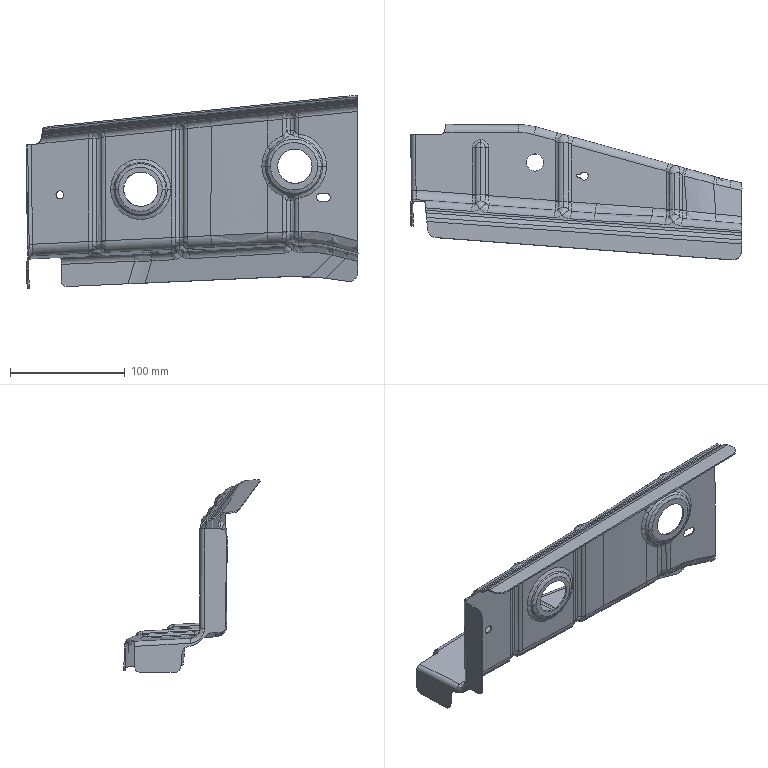Part | 1 solid | 363 faces | box 288.755 x 118.551 x 167.544 mm | volume 77515 mm3 | spline 227 | cylinder 81 | plane 41 | other 6 | sphere 4 | torus 4 | commonest cylinder face diameters 7.6 x14 10 x14 12 x11 14.4 x10 17.6 x5 20 x5